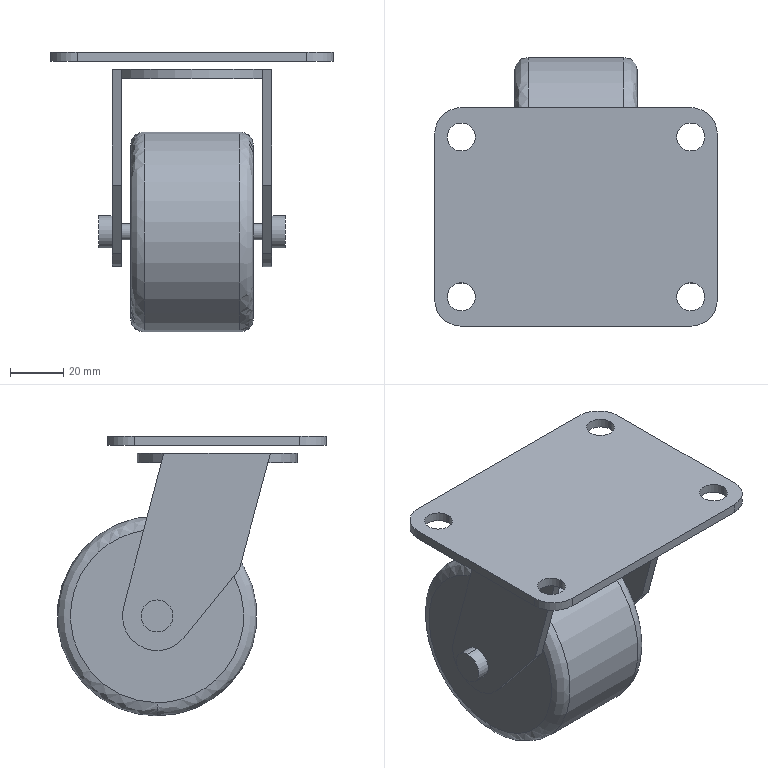Part | SolidWorks | features BaseBody 2 | 2 solids | 59 faces | box 106 x 101 x 105 mm | volume 258638 mm3 | cylinder 31 | plane 24 | spline 4 | commonest cylinder face diameters 10.5 x8 6 x4 8 x4 12 x4 20 x4 26 x3